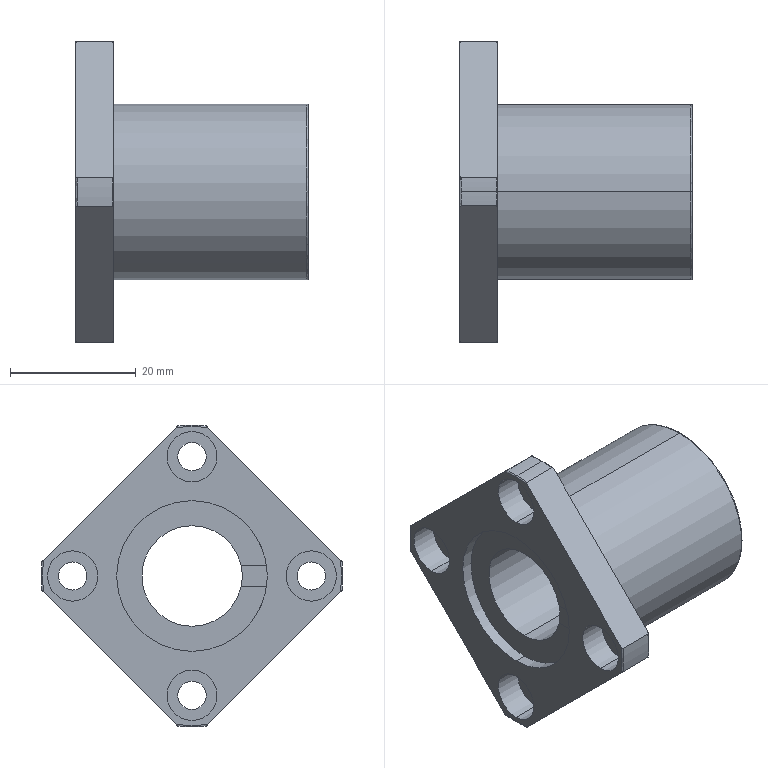Part | STEP file | 1 solid | 60 faces | box 37 x 48 x 48 mm | volume 17828 mm3 | cylinder 29 | plane 19 | spline 12 | commonest cylinder face diameters 4.5 x8 8 x8 48 x5 24 x4 16 x2 28 x2